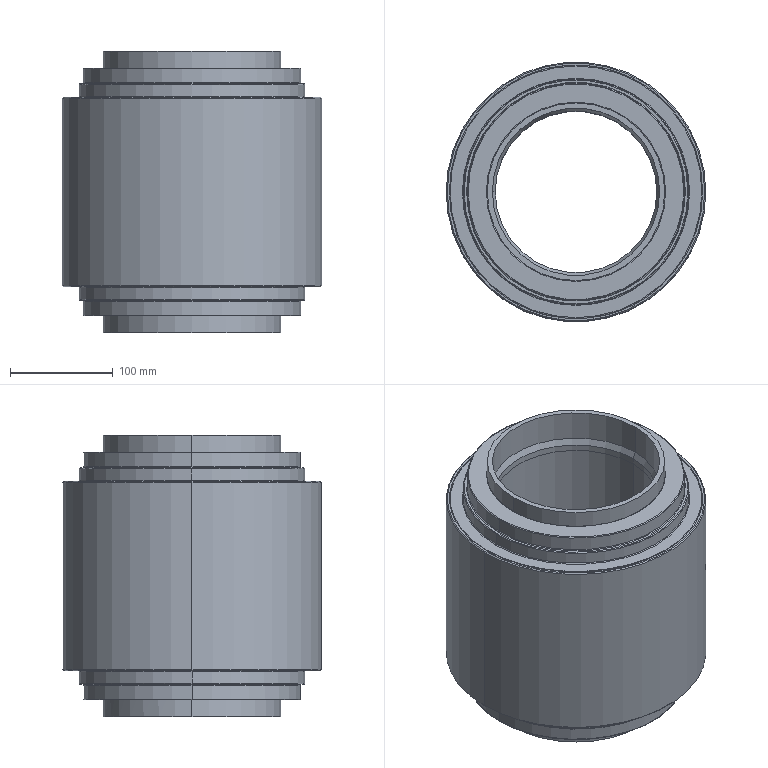Part | SolidWorks | features Revolution 12, CirPattern 2, Fillet 2, Chamfer 1, Cut 1 | 10 solids | 469 faces | box 252.413 x 252.413 x 273.304 mm | volume 4431426 mm3 | cone 340 | cylinder 73 | plane 32 | torus 24 | commonest cylinder face diameters 172.72 x12 157.15 x10 208.25 x8 246.413 x8 162.84 x4 173.15 x4